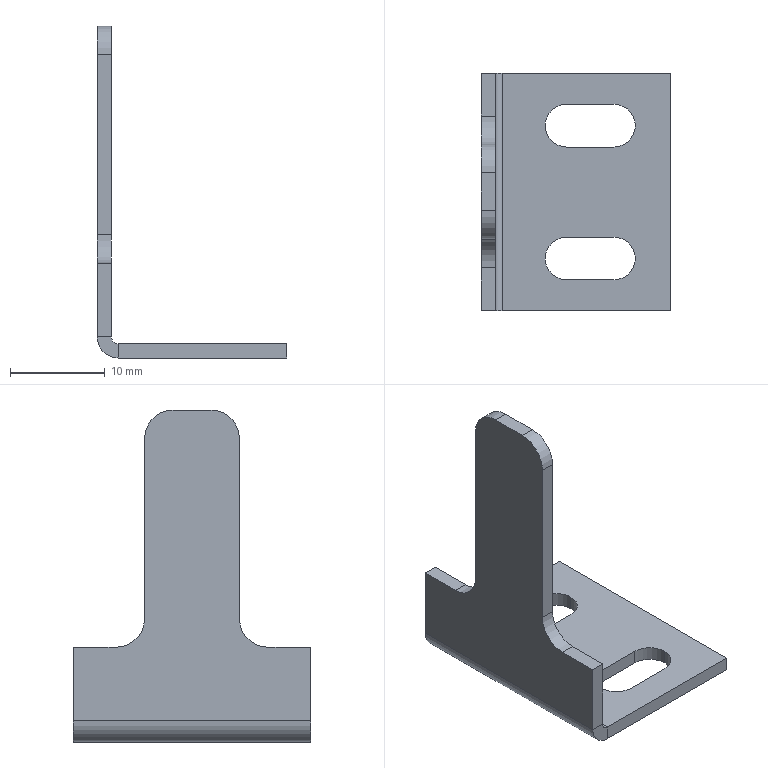Part | SolidWorks | features EdgeFlange 1, Fillet 1, FlatPattern 1, ICE 1, SMBaseFlange 1, SheetMetal 1 | 1 solid | 32 faces | box 20 x 25 x 35 mm | volume 1305 mm3 | plane 20 | cylinder 12 | commonest cylinder face diameters 4.5 x6 6 x4 1.473 x1 4.473 x1
STEP:
#1=CARTESIAN_POINT('',(6.25,-7.,-1.5));
#2=VERTEX_POINT('',#1);
#3=CARTESIAN_POINT('',(4.,-4.75,-1.5));
#4=VERTEX_POINT('',#3);
#5=CARTESIAN_POINT('',(4.,-7.,-1.5));
#6=DIRECTION('',(0.,0.,1.));
#7=DIRECTION('',(1.,0.,0.));
#8=AXIS2_PLACEMENT_3D('',#5,#6,#7);
#9=CIRCLE('',#8,2.25);
#10=EDGE_CURVE('',#2,#4,#9,.T.);
#11=ORIENTED_EDGE('',*,*,#10,.F.);
#12=CARTESIAN_POINT('',(6.25,-7.,0.));
#13=VERTEX_POINT('',#12);
#14=CARTESIAN_POINT('',(6.25,-7.,-1.5));
#15=DIRECTION('',(0.,0.,1.));
#16=VECTOR('',#15,1000.);
#17=LINE('',#14,#16);
#18=EDGE_CURVE('',#2,#13,#17,.T.);
#19=ORIENTED_EDGE('',*,*,#18,.T.);
#20=CARTESIAN_POINT('',(4.,-4.75,0.));
#21=VERTEX_POINT('',#20);
#22=CARTESIAN_POINT('',(4.,-7.,0.));
#23=DIRECTION('',(0.,0.,1.));
#24=DIRECTION('',(1.,0.,0.));
#25=AXIS2_PLACEMENT_3D('',#22,#23,#24);
#26=CIRCLE('',#25,2.25);
#27=EDGE_CURVE('',#13,#21,#26,.T.);
#28=ORIENTED_EDGE('',*,*,#27,.T.);
#29=CARTESIAN_POINT('',(4.,-4.75,-1.5));
#30=DIRECTION('',(0.,0.,1.));
#31=VECTOR('',#30,1000.);
#32=LINE('',#29,#31);
#33=EDGE_CURVE('',#4,#21,#32,.T.);
#34=ORIENTED_EDGE('',*,*,#33,.F.);
#35=EDGE_LOOP('',(#11,#19,#28,#34));
#36=FACE_OUTER_BOUND('',#35,.T.);
#37=CARTESIAN_POINT('',(4.,-7.,-1.5));
#38=DIRECTION('',(0.,0.,1.));
#39=DIRECTION('',(1.,0.,0.));
#40=AXIS2_PLACEMENT_3D('',#37,#38,#39);
#41=CYLINDRICAL_SURFACE('',#40,2.25);
#42=ADVANCED_FACE('',(#36),#41,.F.);
#43=CARTESIAN_POINT('',(6.25,7.,-1.5));
#44=VERTEX_POINT('',#43);
#45=CARTESIAN_POINT('',(4.,9.25,-1.5));
#46=VERTEX_POINT('',#45);
#47=CARTESIAN_POINT('',(4.,7.,-1.5));
#48=DIRECTION('',(0.,0.,1.));
#49=DIRECTION('',(1.,0.,0.));
#50=AXIS2_PLACEMENT_3D('',#47,#48,#49);
#51=CIRCLE('',#50,2.25);
#52=EDGE_CURVE('',#44,#46,#51,.T.);
#53=ORIENTED_EDGE('',*,*,#52,.F.);
#54=CARTESIAN_POINT('',(6.25,7.,0.));
#55=VERTEX_POINT('',#54);
#56=CARTESIAN_POINT('',(6.25,7.,-1.5));
#57=DIRECTION('',(0.,0.,1.));
#58=VECTOR('',#57,1000.);
#59=LINE('',#56,#58);
#60=EDGE_CURVE('',#44,#55,#59,.T.);
#61=ORIENTED_EDGE('',*,*,#60,.T.);
#62=CARTESIAN_POINT('',(4.,9.25,0.));
#63=VERTEX_POINT('',#62);
#64=CARTESIAN_POINT('',(4.,7.,0.));
#65=DIRECTION('',(0.,0.,1.));
#66=DIRECTION('',(1.,0.,0.));
#67=AXIS2_PLACEMENT_3D('',#64,#65,#66);
#68=CIRCLE('',#67,2.25);
#69=EDGE_CURVE('',#55,#63,#68,.T.);
#70=ORIENTED_EDGE('',*,*,#69,.T.);
#71=CARTESIAN_POINT('',(4.,9.25,-1.5));
#72=DIRECTION('',(0.,0.,1.));
#73=VECTOR('',#72,1000.);
#74=LINE('',#71,#73);
#75=EDGE_CURVE('',#46,#63,#74,.T.);
#76=ORIENTED_EDGE('',*,*,#75,.F.);
#77=EDGE_LOOP('',(#53,#61,#70,#76));
#78=FACE_OUTER_BOUND('',#77,.T.);
#79=CARTESIAN_POINT('',(4.,7.,-1.5));
#80=DIRECTION('',(0.,0.,1.));
#81=DIRECTION('',(1.,0.,0.));
#82=AXIS2_PLACEMENT_3D('',#79,#80,#81);
#83=CYLINDRICAL_SURFACE('',#82,2.25);
#84=ADVANCED_FACE('',(#78),#83,.F.);
#85=CARTESIAN_POINT('',(-7.763,-12.5,0.));
#86=VERTEX_POINT('',#85);
#87=CARTESIAN_POINT('',(10.,-12.5,0.));
#88=VERTEX_POINT('',#87);
#89=CARTESIAN_POINT('',(-10.,-12.5,0.));
#90=DIRECTION('',(1.,0.,0.));
#91=VECTOR('',#90,1000.);
#92=LINE('',#89,#91);
#93=EDGE_CURVE('',#86,#88,#92,.T.);
#94=ORIENTED_EDGE('',*,*,#93,.F.);
#95=CARTESIAN_POINT('',(-7.763,-12.5,-1.5));
#96=VERTEX_POINT('',#95);
#97=CARTESIAN_POINT('',(-7.763,-12.5,0.));
#98=DIRECTION('',(0.,0.,-1.));
#99=VECTOR('',#98,1000.);
#100=LINE('',#97,#99);
#101=EDGE_CURVE('',#86,#96,#100,.T.);
#102=ORIENTED_EDGE('',*,*,#101,.T.);
#103=CARTESIAN_POINT('',(10.,-12.5,-1.5));
#104=VERTEX_POINT('',#103);
#105=CARTESIAN_POINT('',(-10.,-12.5,-1.5));
#106=DIRECTION('',(1.,0.,0.));
#107=VECTOR('',#106,1000.);
#108=LINE('',#105,#107);
#109=EDGE_CURVE('',#96,#104,#108,.T.);
#110=ORIENTED_EDGE('',*,*,#109,.T.);
#111=CARTESIAN_POINT('',(10.,-12.5,-1.5));
#112=DIRECTION('',(0.,0.,1.));
#113=VECTOR('',#112,1000.);
#114=LINE('',#111,#113);
#115=EDGE_CURVE('',#104,#88,#114,.T.);
#116=ORIENTED_EDGE('',*,*,#115,.T.);
#117=EDGE_LOOP('',(#94,#102,#110,#116));
#118=FACE_OUTER_BOUND('',#117,.T.);
#119=CARTESIAN_POINT('',(-10.,-12.5,-1.5));
#120=DIRECTION('',(0.,-1.,0.));
#121=DIRECTION('',(0.,0.,-1.));
#122=AXIS2_PLACEMENT_3D('',#119,#120,#121);
#123=PLANE('',#122);
#124=ADVANCED_FACE('',(#118),#123,.T.);
#125=CARTESIAN_POINT('',(-1.,9.25,-1.5));
#126=VERTEX_POINT('',#125);
#127=CARTESIAN_POINT('',(-1.,9.25,-1.5));
#128=DIRECTION('',(-1.,0.,0.));
#129=VECTOR('',#128,1000.);
#130=LINE('',#127,#129);
#131=EDGE_CURVE('',#46,#126,#130,.T.);
#132=ORIENTED_EDGE('',*,*,#131,.T.);
#133=CARTESIAN_POINT('',(-1.,4.75,-1.5));
#134=VERTEX_POINT('',#133);
#135=CARTESIAN_POINT('',(-1.,7.,-1.5));
#136=DIRECTION('',(0.,0.,1.));
#137=DIRECTION('',(1.,0.,0.));
#138=AXIS2_PLACEMENT_3D('',#135,#136,#137);
#139=CIRCLE('',#138,2.25);
#140=EDGE_CURVE('',#126,#134,#139,.T.);
#141=ORIENTED_EDGE('',*,*,#140,.T.);
#142=CARTESIAN_POINT('',(4.,4.75,-1.5));
#143=VERTEX_POINT('',#142);
#144=CARTESIAN_POINT('',(-1.,4.75,-1.5));
#145=DIRECTION('',(1.,0.,0.));
#146=VECTOR('',#145,1000.);
#147=LINE('',#144,#146);
#148=EDGE_CURVE('',#134,#143,#147,.T.);
#149=ORIENTED_EDGE('',*,*,#148,.T.);
#150=CARTESIAN_POINT('',(4.,7.,-1.5));
#151=DIRECTION('',(0.,0.,1.));
#152=DIRECTION('',(1.,0.,0.));
#153=AXIS2_PLACEMENT_3D('',#150,#151,#152);
#154=CIRCLE('',#153,2.25);
#155=EDGE_CURVE('',#143,#44,#154,.T.);
#156=ORIENTED_EDGE('',*,*,#155,.T.);
#157=ORIENTED_EDGE('',*,*,#52,.T.);
#158=EDGE_LOOP('',(#132,#141,#149,#156,#157));
#159=FACE_BOUND('',#158,.T.);
#160=CARTESIAN_POINT('',(-1.,-4.75,-1.5));
#161=VERTEX_POINT('',#160);
#162=CARTESIAN_POINT('',(-1.,-4.75,-1.5));
#163=DIRECTION('',(-1.,0.,0.));
#164=VECTOR('',#163,1000.);
#165=LINE('',#162,#164);
#166=EDGE_CURVE('',#4,#161,#165,.T.);
#167=ORIENTED_EDGE('',*,*,#166,.T.);
#168=CARTESIAN_POINT('',(-1.,-9.25,-1.5));
#169=VERTEX_POINT('',#168);
#170=CARTESIAN_POINT('',(-1.,-7.,-1.5));
#171=DIRECTION('',(0.,0.,1.));
#172=DIRECTION('',(1.,0.,0.));
#173=AXIS2_PLACEMENT_3D('',#170,#171,#172);
#174=CIRCLE('',#173,2.25);
#175=EDGE_CURVE('',#161,#169,#174,.T.);
#176=ORIENTED_EDGE('',*,*,#175,.T.);
#177=CARTESIAN_POINT('',(4.,-9.25,-1.5));
#178=VERTEX_POINT('',#177);
#179=CARTESIAN_POINT('',(-1.,-9.25,-1.5));
#180=DIRECTION('',(1.,0.,0.));
#181=VECTOR('',#180,1000.);
#182=LINE('',#179,#181);
#183=EDGE_CURVE('',#169,#178,#182,.T.);
#184=ORIENTED_EDGE('',*,*,#183,.T.);
#185=CARTESIAN_POINT('',(4.,-7.,-1.5));
#186=DIRECTION('',(0.,0.,1.));
#187=DIRECTION('',(1.,0.,0.));
#188=AXIS2_PLACEMENT_3D('',#185,#186,#187);
#189=CIRCLE('',#188,2.25);
#190=EDGE_CURVE('',#178,#2,#189,.T.);
#191=ORIENTED_EDGE('',*,*,#190,.T.);
#192=ORIENTED_EDGE('',*,*,#10,.T.);
#193=EDGE_LOOP('',(#167,#176,#184,#191,#192));
#194=FACE_BOUND('',#193,.T.);
#195=CARTESIAN_POINT('',(-7.763,12.5,-1.5));
#196=VERTEX_POINT('',#195);
#197=CARTESIAN_POINT('',(-7.763,-12.5,-1.5));
#198=DIRECTION('',(0.,1.,0.));
#199=VECTOR('',#198,1000.);
#200=LINE('',#197,#199);
#201=EDGE_CURVE('',#96,#196,#200,.T.);
#202=ORIENTED_EDGE('',*,*,#201,.T.);
#203=CARTESIAN_POINT('',(10.,12.5,-1.5));
#204=VERTEX_POINT('',#203);
#205=CARTESIAN_POINT('',(-10.,12.5,-1.5));
#206=DIRECTION('',(-1.,0.,0.));
#207=VECTOR('',#206,1000.);
#208=LINE('',#205,#207);
#209=EDGE_CURVE('',#204,#196,#208,.T.);
#210=ORIENTED_EDGE('',*,*,#209,.F.);
#211=CARTESIAN_POINT('',(10.,12.5,-1.5));
#212=DIRECTION('',(0.,1.,0.));
#213=VECTOR('',#212,1000.);
#214=LINE('',#211,#213);
#215=EDGE_CURVE('',#104,#204,#214,.T.);
#216=ORIENTED_EDGE('',*,*,#215,.F.);
#217=ORIENTED_EDGE('',*,*,#109,.F.);
#218=EDGE_LOOP('',(#202,#210,#216,#217));
#219=FACE_OUTER_BOUND('',#218,.T.);
#220=CARTESIAN_POINT('',(0.,0.,-1.5));
#221=DIRECTION('',(0.,0.,1.));
#222=DIRECTION('',(1.,0.,0.));
#223=AXIS2_PLACEMENT_3D('',#220,#221,#222);
#224=PLANE('',#223);
#225=ADVANCED_FACE('',(#159,#194,#219),#224,.F.);
#226=CARTESIAN_POINT('',(-1.,9.25,0.));
#227=VERTEX_POINT('',#226);
#228=CARTESIAN_POINT('',(-1.,4.75,0.));
#229=VERTEX_POINT('',#228);
#230=CARTESIAN_POINT('',(-1.,7.,0.));
#231=DIRECTION('',(0.,0.,1.));
#232=DIRECTION('',(1.,0.,0.));
#233=AXIS2_PLACEMENT_3D('',#230,#231,#232);
#234=CIRCLE('',#233,2.25);
#235=EDGE_CURVE('',#227,#229,#234,.T.);
#236=ORIENTED_EDGE('',*,*,#235,.F.);
#237=CARTESIAN_POINT('',(-1.,9.25,0.));
#238=DIRECTION('',(-1.,0.,0.));
#239=VECTOR('',#238,1000.);
#240=LINE('',#237,#239);
#241=EDGE_CURVE('',#63,#227,#240,.T.);
#242=ORIENTED_EDGE('',*,*,#241,.F.);
#243=ORIENTED_EDGE('',*,*,#69,.F.);
#244=CARTESIAN_POINT('',(4.,4.75,0.));
#245=VERTEX_POINT('',#244);
#246=CARTESIAN_POINT('',(4.,7.,0.));
#247=DIRECTION('',(0.,0.,1.));
#248=DIRECTION('',(1.,0.,0.));
#249=AXIS2_PLACEMENT_3D('',#246,#247,#248);
#250=CIRCLE('',#249,2.25);
#251=EDGE_CURVE('',#245,#55,#250,.T.);
#252=ORIENTED_EDGE('',*,*,#251,.F.);
#253=CARTESIAN_POINT('',(-1.,4.75,0.));
#254=DIRECTION('',(1.,0.,0.));
#255=VECTOR('',#254,1000.);
#256=LINE('',#253,#255);
#257=EDGE_CURVE('',#229,#245,#256,.T.);
#258=ORIENTED_EDGE('',*,*,#257,.F.);
#259=EDGE_LOOP('',(#236,#242,#243,#252,#258));
#260=FACE_BOUND('',#259,.T.);
#261=CARTESIAN_POINT('',(-1.,-4.75,0.));
#262=VERTEX_POINT('',#261);
#263=CARTESIAN_POINT('',(-1.,-9.25,0.));
#264=VERTEX_POINT('',#263);
#265=CARTESIAN_POINT('',(-1.,-7.,0.));
#266=DIRECTION('',(0.,0.,1.));
#267=DIRECTION('',(1.,0.,0.));
#268=AXIS2_PLACEMENT_3D('',#265,#266,#267);
#269=CIRCLE('',#268,2.25);
#270=EDGE_CURVE('',#262,#264,#269,.T.);
#271=ORIENTED_EDGE('',*,*,#270,.F.);
#272=CARTESIAN_POINT('',(-1.,-4.75,0.));
#273=DIRECTION('',(-1.,0.,0.));
#274=VECTOR('',#273,1000.);
#275=LINE('',#272,#274);
#276=EDGE_CURVE('',#21,#262,#275,.T.);
#277=ORIENTED_EDGE('',*,*,#276,.F.);
#278=ORIENTED_EDGE('',*,*,#27,.F.);
#279=CARTESIAN_POINT('',(4.,-9.25,0.));
#280=VERTEX_POINT('',#279);
#281=CARTESIAN_POINT('',(4.,-7.,0.));
#282=DIRECTION('',(0.,0.,1.));
#283=DIRECTION('',(1.,0.,0.));
#284=AXIS2_PLACEMENT_3D('',#281,#282,#283);
#285=CIRCLE('',#284,2.25);
#286=EDGE_CURVE('',#280,#13,#285,.T.);
#287=ORIENTED_EDGE('',*,*,#286,.F.);
#288=CARTESIAN_POINT('',(-1.,-9.25,0.));
#289=DIRECTION('',(1.,0.,0.));
#290=VECTOR('',#289,1000.);
#291=LINE('',#288,#290);
#292=EDGE_CURVE('',#264,#280,#291,.T.);
#293=ORIENTED_EDGE('',*,*,#292,.F.);
#294=EDGE_LOOP('',(#271,#277,#278,#287,#293));
#295=FACE_BOUND('',#294,.T.);
#296=CARTESIAN_POINT('',(10.,12.5,0.));
#297=VERTEX_POINT('',#296);
#298=CARTESIAN_POINT('',(-7.763,12.5,0.));
#299=VERTEX_POINT('',#298);
#300=CARTESIAN_POINT('',(-10.,12.5,0.));
#301=DIRECTION('',(-1.,0.,0.));
#302=VECTOR('',#301,1000.);
#303=LINE('',#300,#302);
#304=EDGE_CURVE('',#297,#299,#303,.T.);
#305=ORIENTED_EDGE('',*,*,#304,.T.);
#306=CARTESIAN_POINT('',(-7.763,-12.5,0.));
#307=DIRECTION('',(0.,1.,0.));
#308=VECTOR('',#307,1000.);
#309=LINE('',#306,#308);
#310=EDGE_CURVE('',#86,#299,#309,.T.);
#311=ORIENTED_EDGE('',*,*,#310,.F.);
#312=ORIENTED_EDGE('',*,*,#93,.T.);
#313=CARTESIAN_POINT('',(10.,12.5,0.));
#314=DIRECTION('',(0.,1.,0.));
#315=VECTOR('',#314,1000.);
#316=LINE('',#313,#315);
#317=EDGE_CURVE('',#88,#297,#316,.T.);
#318=ORIENTED_EDGE('',*,*,#317,.T.);
#319=EDGE_LOOP('',(#305,#311,#312,#318));
#320=FACE_OUTER_BOUND('',#319,.T.);
#321=CARTESIAN_POINT('',(0.,0.,0.));
#322=DIRECTION('',(0.,0.,1.));
#323=DIRECTION('',(1.,0.,0.));
#324=AXIS2_PLACEMENT_3D('',#321,#322,#323);
#325=PLANE('',#324);
#326=ADVANCED_FACE('',(#260,#295,#320),#325,.T.);
#327=ORIENTED_EDGE('',*,*,#317,.F.);
#328=ORIENTED_EDGE('',*,*,#115,.F.);
#329=ORIENTED_EDGE('',*,*,#215,.T.);
#330=CARTESIAN_POINT('',(10.,12.5,-1.5));
#331=DIRECTION('',(0.,0.,1.));
#332=VECTOR('',#331,1000.);
#333=LINE('',#330,#332);
#334=EDGE_CURVE('',#204,#297,#333,.T.);
#335=ORIENTED_EDGE('',*,*,#334,.T.);
#336=EDGE_LOOP('',(#327,#328,#329,#335));
#337=FACE_OUTER_BOUND('',#336,.T.);
#338=CARTESIAN_POINT('',(10.,12.5,-1.5));
#339=DIRECTION('',(1.,0.,0.));
#340=DIRECTION('',(0.,1.,0.));
#341=AXIS2_PLACEMENT_3D('',#338,#339,#340);
#342=PLANE('',#341);
#343=ADVANCED_FACE('',(#337),#342,.T.);
#344=CARTESIAN_POINT('',(-7.763,12.5,0.));
#345=DIRECTION('',(0.,0.,-1.));
#346=VECTOR('',#345,1000.);
#347=LINE('',#344,#346);
#348=EDGE_CURVE('',#299,#196,#347,.T.);
#349=ORIENTED_EDGE('',*,*,#348,.F.);
#350=ORIENTED_EDGE('',*,*,#304,.F.);
#351=ORIENTED_EDGE('',*,*,#334,.F.);
#352=ORIENTED_EDGE('',*,*,#209,.T.);
#353=EDGE_LOOP('',(#349,#350,#351,#352));
#354=FACE_OUTER_BOUND('',#353,.T.);
#355=CARTESIAN_POINT('',(-10.,12.5,-1.5));
#356=DIRECTION('',(0.,1.,0.));
#357=DIRECTION('',(0.,0.,1.));
#358=AXIS2_PLACEMENT_3D('',#355,#356,#357);
#359=PLANE('',#358);
#360=ADVANCED_FACE('',(#354),#359,.T.);
#361=ORIENTED_EDGE('',*,*,#235,.T.);
#362=CARTESIAN_POINT('',(-1.,4.75,-1.5));
#363=DIRECTION('',(0.,0.,1.));
#364=VECTOR('',#363,1000.);
#365=LINE('',#362,#364);
#366=EDGE_CURVE('',#134,#229,#365,.T.);
#367=ORIENTED_EDGE('',*,*,#366,.F.);
#368=ORIENTED_EDGE('',*,*,#140,.F.);
#369=CARTESIAN_POINT('',(-1.,9.25,-1.5));
#370=DIRECTION('',(0.,0.,1.));
#371=VECTOR('',#370,1000.);
#372=LINE('',#369,#371);
#373=EDGE_CURVE('',#126,#227,#372,.T.);
#374=ORIENTED_EDGE('',*,*,#373,.T.);
#375=EDGE_LOOP('',(#361,#367,#368,#374));
#376=FACE_OUTER_BOUND('',#375,.T.);
#377=CARTESIAN_POINT('',(-1.,7.,-1.5));
#378=DIRECTION('',(0.,0.,1.));
#379=DIRECTION('',(1.,0.,0.));
#380=AXIS2_PLACEMENT_3D('',#377,#378,#379);
#381=CYLINDRICAL_SURFACE('',#380,2.25);
#382=ADVANCED_FACE('',(#376),#381,.F.);
#383=ORIENTED_EDGE('',*,*,#241,.T.);
#384=ORIENTED_EDGE('',*,*,#373,.F.);
#385=ORIENTED_EDGE('',*,*,#131,.F.);
#386=ORIENTED_EDGE('',*,*,#75,.T.);
#387=EDGE_LOOP('',(#383,#384,#385,#386));
#388=FACE_OUTER_BOUND('',#387,.T.);
#389=CARTESIAN_POINT('',(-1.,9.25,-1.5));
#390=DIRECTION('',(0.,1.,0.));
#391=DIRECTION('',(0.,0.,1.));
#392=AXIS2_PLACEMENT_3D('',#389,#390,#391);
#393=PLANE('',#392);
#394=ADVANCED_FACE('',(#388),#393,.F.);
#395=ORIENTED_EDGE('',*,*,#60,.F.);
#396=ORIENTED_EDGE('',*,*,#155,.F.);
#397=CARTESIAN_POINT('',(4.,4.75,-1.5));
#398=DIRECTION('',(0.,0.,1.));
#399=VECTOR('',#398,1000.);
#400=LINE('',#397,#399);
#401=EDGE_CURVE('',#143,#245,#400,.T.);
#402=ORIENTED_EDGE('',*,*,#401,.T.);
#403=ORIENTED_EDGE('',*,*,#251,.T.);
#404=EDGE_LOOP('',(#395,#396,#402,#403));
#405=FACE_OUTER_BOUND('',#404,.T.);
#406=CARTESIAN_POINT('',(4.,7.,-1.5));
#407=DIRECTION('',(0.,0.,1.));
#408=DIRECTION('',(1.,0.,0.));
#409=AXIS2_PLACEMENT_3D('',#406,#407,#408);
#410=CYLINDRICAL_SURFACE('',#409,2.25);
#411=ADVANCED_FACE('',(#405),#410,.F.);
#412=ORIENTED_EDGE('',*,*,#257,.T.);
#413=ORIENTED_EDGE('',*,*,#401,.F.);
#414=ORIENTED_EDGE('',*,*,#148,.F.);
#415=ORIENTED_EDGE('',*,*,#366,.T.);
#416=EDGE_LOOP('',(#412,#413,#414,#415));
#417=FACE_OUTER_BOUND('',#416,.T.);
#418=CARTESIAN_POINT('',(-1.,4.75,-1.5));
#419=DIRECTION('',(0.,-1.,0.));
#420=DIRECTION('',(0.,0.,-1.));
#421=AXIS2_PLACEMENT_3D('',#418,#419,#420);
#422=PLANE('',#421);
#423=ADVANCED_FACE('',(#417),#422,.F.);
#424=ORIENTED_EDGE('',*,*,#270,.T.);
#425=CARTESIAN_POINT('',(-1.,-9.25,-1.5));
#426=DIRECTION('',(0.,0.,1.));
#427=VECTOR('',#426,1000.);
#428=LINE('',#425,#427);
#429=EDGE_CURVE('',#169,#264,#428,.T.);
#430=ORIENTED_EDGE('',*,*,#429,.F.);
#431=ORIENTED_EDGE('',*,*,#175,.F.);
#432=CARTESIAN_POINT('',(-1.,-4.75,-1.5));
#433=DIRECTION('',(0.,0.,1.));
#434=VECTOR('',#433,1000.);
#435=LINE('',#432,#434);
#436=EDGE_CURVE('',#161,#262,#435,.T.);
#437=ORIENTED_EDGE('',*,*,#436,.T.);
#438=EDGE_LOOP('',(#424,#430,#431,#437));
#439=FACE_OUTER_BOUND('',#438,.T.);
#440=CARTESIAN_POINT('',(-1.,-7.,-1.5));
#441=DIRECTION('',(0.,0.,1.));
#442=DIRECTION('',(1.,0.,0.));
#443=AXIS2_PLACEMENT_3D('',#440,#441,#442);
#444=CYLINDRICAL_SURFACE('',#443,2.25);
#445=ADVANCED_FACE('',(#439),#444,.F.);
#446=ORIENTED_EDGE('',*,*,#276,.T.);
#447=ORIENTED_EDGE('',*,*,#436,.F.);
#448=ORIENTED_EDGE('',*,*,#166,.F.);
#449=ORIENTED_EDGE('',*,*,#33,.T.);
#450=EDGE_LOOP('',(#446,#447,#448,#449));
#451=FACE_OUTER_BOUND('',#450,.T.);
#452=CARTESIAN_POINT('',(-1.,-4.75,-1.5));
#453=DIRECTION('',(0.,1.,0.));
#454=DIRECTION('',(0.,0.,1.));
#455=AXIS2_PLACEMENT_3D('',#452,#453,#454);
#456=PLANE('',#455);
#457=ADVANCED_FACE('',(#451),#456,.F.);
#458=ORIENTED_EDGE('',*,*,#18,.F.);
#459=ORIENTED_EDGE('',*,*,#190,.F.);
#460=CARTESIAN_POINT('',(4.,-9.25,-1.5));
#461=DIRECTION('',(0.,0.,1.));
#462=VECTOR('',#461,1000.);
#463=LINE('',#460,#462);
#464=EDGE_CURVE('',#178,#280,#463,.T.);
#465=ORIENTED_EDGE('',*,*,#464,.T.);
#466=ORIENTED_EDGE('',*,*,#286,.T.);
#467=EDGE_LOOP('',(#458,#459,#465,#466));
#468=FACE_OUTER_BOUND('',#467,.T.);
#469=CARTESIAN_POINT('',(4.,-7.,-1.5));
#470=DIRECTION('',(0.,0.,1.));
#471=DIRECTION('',(1.,0.,0.));
#472=AXIS2_PLACEMENT_3D('',#469,#470,#471);
#473=CYLINDRICAL_SURFACE('',#472,2.25);
#474=ADVANCED_FACE('',(#468),#473,.F.);
#475=ORIENTED_EDGE('',*,*,#292,.T.);
#476=ORIENTED_EDGE('',*,*,#464,.F.);
#477=ORIENTED_EDGE('',*,*,#183,.F.);
#478=ORIENTED_EDGE('',*,*,#429,.T.);
#479=EDGE_LOOP('',(#475,#476,#477,#478));
#480=FACE_OUTER_BOUND('',#479,.T.);
#481=CARTESIAN_POINT('',(-1.,-9.25,-1.5));
#482=DIRECTION('',(0.,-1.,0.));
#483=DIRECTION('',(0.,0.,-1.));
#484=AXIS2_PLACEMENT_3D('',#481,#482,#483);
#485=PLANE('',#484);
#486=ADVANCED_FACE('',(#480),#485,.F.);
#487=CARTESIAN_POINT('',(-8.5,12.5,0.7366));
#488=VERTEX_POINT('',#487);
#489=CARTESIAN_POINT('',(-10.,12.5,0.7366));
#490=VERTEX_POINT('',#489);
#491=CARTESIAN_POINT('',(-10.,12.5,0.7366));
#492=DIRECTION('',(-1.,0.,0.));
#493=VECTOR('',#492,1000.);
#494=LINE('',#491,#493);
#495=EDGE_CURVE('',#488,#490,#494,.T.);
#496=ORIENTED_EDGE('',*,*,#495,.F.);
#497=CARTESIAN_POINT('',(-7.763,12.5,0.7366));
#498=DIRECTION('',(0.,1.,0.));
#499=DIRECTION('',(0.,0.,-1.));
#500=AXIS2_PLACEMENT_3D('',#497,#498,#499);
#501=CIRCLE('',#500,0.7366);
#502=EDGE_CURVE('',#299,#488,#501,.T.);
#503=ORIENTED_EDGE('',*,*,#502,.F.);
#504=ORIENTED_EDGE('',*,*,#348,.T.);
#505=CARTESIAN_POINT('',(-7.763,12.5,0.7366));
#506=DIRECTION('',(0.,1.,0.));
#507=DIRECTION('',(0.,0.,-1.));
#508=AXIS2_PLACEMENT_3D('',#505,#506,#507);
#509=CIRCLE('',#508,2.237);
#510=EDGE_CURVE('',#196,#490,#509,.T.);
#511=ORIENTED_EDGE('',*,*,#510,.T.);
#512=EDGE_LOOP('',(#496,#503,#504,#511));
#513=FACE_OUTER_BOUND('',#512,.T.);
#514=CARTESIAN_POINT('',(-7.763,12.5,0.7366));
#515=DIRECTION('',(0.,1.,0.));
#516=DIRECTION('',(0.,0.,1.));
#517=AXIS2_PLACEMENT_3D('',#514,#515,#516);
#518=PLANE('',#517);
#519=ADVANCED_FACE('',(#513),#518,.T.);
#520=CARTESIAN_POINT('',(-8.5,-12.5,0.7366));
#521=VERTEX_POINT('',#520);
#522=CARTESIAN_POINT('',(-7.763,-12.5,0.7366));
#523=DIRECTION('',(0.,-1.,0.));
#524=DIRECTION('',(0.,0.,-1.));
#525=AXIS2_PLACEMENT_3D('',#522,#523,#524);
#526=CIRCLE('',#525,0.7366);
#527=EDGE_CURVE('',#521,#86,#526,.T.);
#528=ORIENTED_EDGE('',*,*,#527,.F.);
#529=CARTESIAN_POINT('',(-10.,-12.5,0.7366));
#530=VERTEX_POINT('',#529);
#531=CARTESIAN_POINT('',(-8.5,-12.5,0.7366));
#532=DIRECTION('',(-1.,0.,0.));
#533=VECTOR('',#532,1000.);
#534=LINE('',#531,#533);
#535=EDGE_CURVE('',#521,#530,#534,.T.);
#536=ORIENTED_EDGE('',*,*,#535,.T.);
#537=CARTESIAN_POINT('',(-7.763,-12.5,0.7366));
#538=DIRECTION('',(0.,-1.,0.));
#539=DIRECTION('',(0.,0.,-1.));
#540=AXIS2_PLACEMENT_3D('',#537,#538,#539);
#541=CIRCLE('',#540,2.237);
#542=EDGE_CURVE('',#530,#96,#541,.T.);
#543=ORIENTED_EDGE('',*,*,#542,.T.);
#544=ORIENTED_EDGE('',*,*,#101,.F.);
#545=EDGE_LOOP('',(#528,#536,#543,#544));
#546=FACE_OUTER_BOUND('',#545,.T.);
#547=CARTESIAN_POINT('',(-7.763,-12.5,0.7366));
#548=DIRECTION('',(0.,1.,0.));
#549=DIRECTION('',(0.,0.,1.));
#550=AXIS2_PLACEMENT_3D('',#547,#548,#549);
#551=PLANE('',#550);
#552=ADVANCED_FACE('',(#546),#551,.F.);
#553=ORIENTED_EDGE('',*,*,#201,.F.);
#554=ORIENTED_EDGE('',*,*,#542,.F.);
#555=CARTESIAN_POINT('',(-10.,12.5,0.7366));
#556=DIRECTION('',(0.,1.,0.));
#557=VECTOR('',#556,1000.);
#558=LINE('',#555,#557);
#559=EDGE_CURVE('',#530,#490,#558,.T.);
#560=ORIENTED_EDGE('',*,*,#559,.T.);
#561=ORIENTED_EDGE('',*,*,#510,.F.);
#562=EDGE_LOOP('',(#553,#554,#560,#561));
#563=FACE_OUTER_BOUND('',#562,.T.);
#564=CARTESIAN_POINT('',(-7.763,-12.5,0.7366));
#565=DIRECTION('',(0.,-1.,0.));
#566=DIRECTION('',(-1.,0.,0.));
#567=AXIS2_PLACEMENT_3D('',#564,#565,#566);
#568=CYLINDRICAL_SURFACE('',#567,2.237);
#569=ADVANCED_FACE('',(#563),#568,.T.);
#570=ORIENTED_EDGE('',*,*,#310,.T.);
#571=ORIENTED_EDGE('',*,*,#502,.T.);
#572=CARTESIAN_POINT('',(-8.5,12.5,0.7366));
#573=DIRECTION('',(0.,-1.,0.));
#574=VECTOR('',#573,1000.);
#575=LINE('',#572,#574);
#576=EDGE_CURVE('',#488,#521,#575,.T.);
#577=ORIENTED_EDGE('',*,*,#576,.T.);
#578=ORIENTED_EDGE('',*,*,#527,.T.);
#579=EDGE_LOOP('',(#570,#571,#577,#578));
#580=FACE_OUTER_BOUND('',#579,.T.);
#581=CARTESIAN_POINT('',(-7.763,-12.5,0.7366));
#582=DIRECTION('',(0.,-1.,0.));
#583=DIRECTION('',(-1.,0.,0.));
#584=AXIS2_PLACEMENT_3D('',#581,#582,#583);
#585=CYLINDRICAL_SURFACE('',#584,0.7366);
#586=ADVANCED_FACE('',(#580),#585,.F.);
#587=CARTESIAN_POINT('',(-10.,12.5,8.5));
#588=VERTEX_POINT('',#587);
#589=CARTESIAN_POINT('',(-10.,12.5,0.));
#590=DIRECTION('',(0.,0.,-1.));
#591=VECTOR('',#590,1000.);
#592=LINE('',#589,#591);
#593=EDGE_CURVE('',#588,#490,#592,.T.);
#594=ORIENTED_EDGE('',*,*,#593,.F.);
#595=CARTESIAN_POINT('',(-8.5,12.5,8.5));
#596=VERTEX_POINT('',#595);
#597=CARTESIAN_POINT('',(0.,12.5,8.5));
#598=DIRECTION('',(-1.,0.,0.));
#599=VECTOR('',#598,1000.);
#600=LINE('',#597,#599);
#601=EDGE_CURVE('',#596,#588,#600,.T.);
#602=ORIENTED_EDGE('',*,*,#601,.F.);
#603=CARTESIAN_POINT('',(-8.5,12.5,0.));
#604=DIRECTION('',(0.,0.,-1.));
#605=VECTOR('',#604,1000.);
#606=LINE('',#603,#605);
#607=EDGE_CURVE('',#596,#488,#606,.T.);
#608=ORIENTED_EDGE('',*,*,#607,.T.);
#609=ORIENTED_EDGE('',*,*,#495,.T.);
#610=EDGE_LOOP('',(#594,#602,#608,#609));
#611=FACE_OUTER_BOUND('',#610,.T.);
#612=CARTESIAN_POINT('',(-10.,12.5,0.));
#613=DIRECTION('',(0.,-1.,0.));
#614=DIRECTION('',(1.,0.,0.));
#615=AXIS2_PLACEMENT_3D('',#612,#613,#614);
#616=PLANE('',#615);
#617=ADVANCED_FACE('',(#611),#616,.F.);
#618=CARTESIAN_POINT('',(-8.5,-12.5,8.5));
#619=VERTEX_POINT('',#618);
#620=CARTESIAN_POINT('',(-8.5,-12.5,33.5));
#621=DIRECTION('',(0.,0.,1.));
#622=VECTOR('',#621,1000.);
#623=LINE('',#620,#622);
#624=EDGE_CURVE('',#521,#619,#623,.T.);
#625=ORIENTED_EDGE('',*,*,#624,.T.);
#626=CARTESIAN_POINT('',(-10.,-12.5,8.5));
#627=VERTEX_POINT('',#626);
#628=CARTESIAN_POINT('',(0.,-12.5,8.5));
#629=DIRECTION('',(-1.,0.,0.));
#630=VECTOR('',#629,1000.);
#631=LINE('',#628,#630);
#632=EDGE_CURVE('',#619,#627,#631,.T.);
#633=ORIENTED_EDGE('',*,*,#632,.T.);
#634=CARTESIAN_POINT('',(-10.,-12.5,0.));
#635=DIRECTION('',(0.,0.,1.));
#636=VECTOR('',#635,1000.);
#637=LINE('',#634,#636);
#638=EDGE_CURVE('',#530,#627,#637,.T.);
#639=ORIENTED_EDGE('',*,*,#638,.F.);
#640=ORIENTED_EDGE('',*,*,#535,.F.);
#641=EDGE_LOOP('',(#625,#633,#639,#640));
#642=FACE_OUTER_BOUND('',#641,.T.);
#643=CARTESIAN_POINT('',(-10.,-12.5,33.5));
#644=DIRECTION('',(0.,1.,0.));
#645=DIRECTION('',(-1.,0.,0.));
#646=AXIS2_PLACEMENT_3D('',#643,#644,#645);
#647=PLANE('',#646);
#648=ADVANCED_FACE('',(#642),#647,.F.);
#649=CARTESIAN_POINT('',(-10.,-2.,33.5));
#650=VERTEX_POINT('',#649);
#651=CARTESIAN_POINT('',(-10.,2.,33.5));
#652=VERTEX_POINT('',#651);
#653=CARTESIAN_POINT('',(-10.,0.,33.5));
#654=DIRECTION('',(0.,1.,0.));
#655=VECTOR('',#654,1000.);
#656=LINE('',#653,#655);
#657=EDGE_CURVE('',#650,#652,#656,.T.);
#658=ORIENTED_EDGE('',*,*,#657,.T.);
#659=CARTESIAN_POINT('',(-10.,5.,30.5));
#660=VERTEX_POINT('',#659);
#661=CARTESIAN_POINT('',(-10.,2.,30.5));
#662=DIRECTION('',(-1.,0.,0.));
#663=DIRECTION('',(0.,0.,-1.));
#664=AXIS2_PLACEMENT_3D('',#661,#662,#663);
#665=CIRCLE('',#664,3.);
#666=EDGE_CURVE('',#652,#660,#665,.T.);
#667=ORIENTED_EDGE('',*,*,#666,.T.);
#668=CARTESIAN_POINT('',(-10.,5.,11.5));
#669=VERTEX_POINT('',#668);
#670=CARTESIAN_POINT('',(-10.,5.,33.5));
#671=DIRECTION('',(0.,0.,1.));
#672=VECTOR('',#671,1000.);
#673=LINE('',#670,#672);
#674=EDGE_CURVE('',#669,#660,#673,.T.);
#675=ORIENTED_EDGE('',*,*,#674,.F.);
#676=CARTESIAN_POINT('',(-10.,8.,8.5));
#677=VERTEX_POINT('',#676);
#678=CARTESIAN_POINT('',(-10.,8.,11.5));
#679=DIRECTION('',(1.,0.,0.));
#680=DIRECTION('',(0.,0.,-1.));
#681=AXIS2_PLACEMENT_3D('',#678,#679,#680);
#682=CIRCLE('',#681,3.);
#683=EDGE_CURVE('',#669,#677,#682,.T.);
#684=ORIENTED_EDGE('',*,*,#683,.T.);
#685=CARTESIAN_POINT('',(-10.,12.5,8.5));
#686=DIRECTION('',(0.,-1.,0.));
#687=VECTOR('',#686,1000.);
#688=LINE('',#685,#687);
#689=EDGE_CURVE('',#588,#677,#688,.T.);
#690=ORIENTED_EDGE('',*,*,#689,.F.);
#691=ORIENTED_EDGE('',*,*,#593,.T.);
#692=ORIENTED_EDGE('',*,*,#559,.F.);
#693=ORIENTED_EDGE('',*,*,#638,.T.);
#694=CARTESIAN_POINT('',(-10.,-8.,8.5));
#695=VERTEX_POINT('',#694);
#696=CARTESIAN_POINT('',(-10.,-12.5,8.5));
#697=DIRECTION('',(0.,-1.,0.));
#698=VECTOR('',#697,1000.);
#699=LINE('',#696,#698);
#700=EDGE_CURVE('',#695,#627,#699,.T.);
#701=ORIENTED_EDGE('',*,*,#700,.F.);
#702=CARTESIAN_POINT('',(-10.,-5.,11.5));
#703=VERTEX_POINT('',#702);
#704=CARTESIAN_POINT('',(-10.,-8.,11.5));
#705=DIRECTION('',(1.,0.,0.));
#706=DIRECTION('',(0.,0.,-1.));
#707=AXIS2_PLACEMENT_3D('',#704,#705,#706);
#708=CIRCLE('',#707,3.);
#709=EDGE_CURVE('',#695,#703,#708,.T.);
#710=ORIENTED_EDGE('',*,*,#709,.T.);
#711=CARTESIAN_POINT('',(-10.,-5.,30.5));
#712=VERTEX_POINT('',#711);
#713=CARTESIAN_POINT('',(-10.,-5.,33.5));
#714=DIRECTION('',(0.,0.,-1.));
#715=VECTOR('',#714,1000.);
#716=LINE('',#713,#715);
#717=EDGE_CURVE('',#712,#703,#716,.T.);
#718=ORIENTED_EDGE('',*,*,#717,.F.);
#719=CARTESIAN_POINT('',(-10.,-2.,30.5));
#720=DIRECTION('',(-1.,0.,0.));
#721=DIRECTION('',(0.,0.,-1.));
#722=AXIS2_PLACEMENT_3D('',#719,#720,#721);
#723=CIRCLE('',#722,3.);
#724=EDGE_CURVE('',#712,#650,#723,.T.);
#725=ORIENTED_EDGE('',*,*,#724,.T.);
#726=EDGE_LOOP('',(#658,#667,#675,#684,#690,#691,#692,#693,#701,#710,#718,#725));
#727=FACE_OUTER_BOUND('',#726,.T.);
#728=CARTESIAN_POINT('',(-10.,0.,0.));
#729=DIRECTION('',(1.,0.,0.));
#730=DIRECTION('',(0.,0.,-1.));
#731=AXIS2_PLACEMENT_3D('',#728,#729,#730);
#732=PLANE('',#731);
#733=ADVANCED_FACE('',(#727),#732,.F.);
#734=CARTESIAN_POINT('',(-8.5,5.,30.5));
#735=VERTEX_POINT('',#734);
#736=CARTESIAN_POINT('',(-8.5,5.,11.5));
#737=VERTEX_POINT('',#736);
#738=CARTESIAN_POINT('',(-8.5,5.,0.));
#739=DIRECTION('',(0.,0.,-1.));
#740=VECTOR('',#739,1000.);
#741=LINE('',#738,#740);
#742=EDGE_CURVE('',#735,#737,#741,.T.);
#743=ORIENTED_EDGE('',*,*,#742,.F.);
#744=CARTESIAN_POINT('',(-8.5,2.,33.5));
#745=VERTEX_POINT('',#744);
#746=CARTESIAN_POINT('',(-8.5,2.,30.5));
#747=DIRECTION('',(1.,0.,0.));
#748=DIRECTION('',(0.,0.,-1.));
#749=AXIS2_PLACEMENT_3D('',#746,#747,#748);
#750=CIRCLE('',#749,3.);
#751=EDGE_CURVE('',#735,#745,#750,.T.);
#752=ORIENTED_EDGE('',*,*,#751,.T.);
#753=CARTESIAN_POINT('',(-8.5,-2.,33.5));
#754=VERTEX_POINT('',#753);
#755=CARTESIAN_POINT('',(-8.5,12.5,33.5));
#756=DIRECTION('',(0.,1.,0.));
#757=VECTOR('',#756,1000.);
#758=LINE('',#755,#757);
#759=EDGE_CURVE('',#754,#745,#758,.T.);
#760=ORIENTED_EDGE('',*,*,#759,.F.);
#761=CARTESIAN_POINT('',(-8.5,-5.,30.5));
#762=VERTEX_POINT('',#761);
#763=CARTESIAN_POINT('',(-8.5,-2.,30.5));
#764=DIRECTION('',(1.,0.,0.));
#765=DIRECTION('',(0.,0.,-1.));
#766=AXIS2_PLACEMENT_3D('',#763,#764,#765);
#767=CIRCLE('',#766,3.);
#768=EDGE_CURVE('',#754,#762,#767,.T.);
#769=ORIENTED_EDGE('',*,*,#768,.T.);
#770=CARTESIAN_POINT('',(-8.5,-5.,11.5));
#771=VERTEX_POINT('',#770);
#772=CARTESIAN_POINT('',(-8.5,-5.,0.));
#773=DIRECTION('',(0.,0.,1.));
#774=VECTOR('',#773,1000.);
#775=LINE('',#772,#774);
#776=EDGE_CURVE('',#771,#762,#775,.T.);
#777=ORIENTED_EDGE('',*,*,#776,.F.);
#778=CARTESIAN_POINT('',(-8.5,-8.,8.5));
#779=VERTEX_POINT('',#778);
#780=CARTESIAN_POINT('',(-8.5,-8.,11.5));
#781=DIRECTION('',(-1.,0.,0.));
#782=DIRECTION('',(0.,0.,-1.));
#783=AXIS2_PLACEMENT_3D('',#780,#781,#782);
#784=CIRCLE('',#783,3.);
#785=EDGE_CURVE('',#771,#779,#784,.T.);
#786=ORIENTED_EDGE('',*,*,#785,.T.);
#787=CARTESIAN_POINT('',(-8.5,0.,8.5));
#788=DIRECTION('',(0.,1.,0.));
#789=VECTOR('',#788,1000.);
#790=LINE('',#787,#789);
#791=EDGE_CURVE('',#619,#779,#790,.T.);
#792=ORIENTED_EDGE('',*,*,#791,.F.);
#793=ORIENTED_EDGE('',*,*,#624,.F.);
#794=ORIENTED_EDGE('',*,*,#576,.F.);
#795=ORIENTED_EDGE('',*,*,#607,.F.);
#796=CARTESIAN_POINT('',(-8.5,8.,8.5));
#797=VERTEX_POINT('',#796);
#798=CARTESIAN_POINT('',(-8.5,0.,8.5));
#799=DIRECTION('',(0.,1.,0.));
#800=VECTOR('',#799,1000.);
#801=LINE('',#798,#800);
#802=EDGE_CURVE('',#797,#596,#801,.T.);
#803=ORIENTED_EDGE('',*,*,#802,.F.);
#804=CARTESIAN_POINT('',(-8.5,8.,11.5));
#805=DIRECTION('',(-1.,0.,0.));
#806=DIRECTION('',(0.,0.,-1.));
#807=AXIS2_PLACEMENT_3D('',#804,#805,#806);
#808=CIRCLE('',#807,3.);
#809=EDGE_CURVE('',#797,#737,#808,.T.);
#810=ORIENTED_EDGE('',*,*,#809,.T.);
#811=EDGE_LOOP('',(#743,#752,#760,#769,#777,#786,#792,#793,#794,#795,#803,#810));
#812=FACE_OUTER_BOUND('',#811,.T.);
#813=CARTESIAN_POINT('',(-8.5,0.,0.));
#814=DIRECTION('',(1.,0.,0.));
#815=DIRECTION('',(0.,0.,-1.));
#816=AXIS2_PLACEMENT_3D('',#813,#814,#815);
#817=PLANE('',#816);
#818=ADVANCED_FACE('',(#812),#817,.T.);
#819=ORIENTED_EDGE('',*,*,#759,.T.);
#820=CARTESIAN_POINT('',(-10.,2.,33.5));
#821=DIRECTION('',(-1.,0.,0.));
#822=VECTOR('',#821,1000.);
#823=LINE('',#820,#822);
#824=EDGE_CURVE('',#745,#652,#823,.T.);
#825=ORIENTED_EDGE('',*,*,#824,.T.);
#826=ORIENTED_EDGE('',*,*,#657,.F.);
#827=CARTESIAN_POINT('',(-10.,-2.,33.5));
#828=DIRECTION('',(1.,0.,0.));
#829=VECTOR('',#828,1000.);
#830=LINE('',#827,#829);
#831=EDGE_CURVE('',#650,#754,#830,.T.);
#832=ORIENTED_EDGE('',*,*,#831,.T.);
#833=EDGE_LOOP('',(#819,#825,#826,#832));
#834=FACE_OUTER_BOUND('',#833,.T.);
#835=CARTESIAN_POINT('',(-10.,12.5,33.5));
#836=DIRECTION('',(0.,0.,-1.));
#837=DIRECTION('',(-1.,0.,0.));
#838=AXIS2_PLACEMENT_3D('',#835,#836,#837);
#839=PLANE('',#838);
#840=ADVANCED_FACE('',(#834),#839,.F.);
#841=ORIENTED_EDGE('',*,*,#674,.T.);
#842=CARTESIAN_POINT('',(0.,5.,30.5));
#843=DIRECTION('',(1.,0.,0.));
#844=VECTOR('',#843,1000.);
#845=LINE('',#842,#844);
#846=EDGE_CURVE('',#660,#735,#845,.T.);
#847=ORIENTED_EDGE('',*,*,#846,.T.);
#848=ORIENTED_EDGE('',*,*,#742,.T.);
#849=CARTESIAN_POINT('',(-10.,5.,11.5));
#850=DIRECTION('',(-1.,0.,0.));
#851=VECTOR('',#850,1000.);
#852=LINE('',#849,#851);
#853=EDGE_CURVE('',#737,#669,#852,.T.);
#854=ORIENTED_EDGE('',*,*,#853,.T.);
#855=EDGE_LOOP('',(#841,#847,#848,#854));
#856=FACE_OUTER_BOUND('',#855,.T.);
#857=CARTESIAN_POINT('',(0.,5.,33.5));
#858=DIRECTION('',(0.,-1.,0.));
#859=DIRECTION('',(1.,0.,0.));
#860=AXIS2_PLACEMENT_3D('',#857,#858,#859);
#861=PLANE('',#860);
#862=ADVANCED_FACE('',(#856),#861,.F.);
#863=ORIENTED_EDGE('',*,*,#689,.T.);
#864=CARTESIAN_POINT('',(-8.5,8.,8.5));
#865=DIRECTION('',(1.,0.,0.));
#866=VECTOR('',#865,1000.);
#867=LINE('',#864,#866);
#868=EDGE_CURVE('',#677,#797,#867,.T.);
#869=ORIENTED_EDGE('',*,*,#868,.T.);
#870=ORIENTED_EDGE('',*,*,#802,.T.);
#871=ORIENTED_EDGE('',*,*,#601,.T.);
#872=EDGE_LOOP('',(#863,#869,#870,#871));
#873=FACE_OUTER_BOUND('',#872,.T.);
#874=CARTESIAN_POINT('',(0.,12.5,8.5));
#875=DIRECTION('',(0.,0.,-1.));
#876=DIRECTION('',(-1.,0.,0.));
#877=AXIS2_PLACEMENT_3D('',#874,#875,#876);
#878=PLANE('',#877);
#879=ADVANCED_FACE('',(#873),#878,.F.);
#880=ORIENTED_EDGE('',*,*,#791,.T.);
#881=CARTESIAN_POINT('',(-10.,-8.,8.5));
#882=DIRECTION('',(-1.,0.,0.));
#883=VECTOR('',#882,1000.);
#884=LINE('',#881,#883);
#885=EDGE_CURVE('',#779,#695,#884,.T.);
#886=ORIENTED_EDGE('',*,*,#885,.T.);
#887=ORIENTED_EDGE('',*,*,#700,.T.);
#888=ORIENTED_EDGE('',*,*,#632,.F.);
#889=EDGE_LOOP('',(#880,#886,#887,#888));
#890=FACE_OUTER_BOUND('',#889,.T.);
#891=CARTESIAN_POINT('',(0.,-12.5,8.5));
#892=DIRECTION('',(0.,0.,-1.));
#893=DIRECTION('',(-1.,0.,0.));
#894=AXIS2_PLACEMENT_3D('',#891,#892,#893);
#895=PLANE('',#894);
#896=ADVANCED_FACE('',(#890),#895,.F.);
#897=ORIENTED_EDGE('',*,*,#776,.T.);
#898=CARTESIAN_POINT('',(0.,-5.,30.5));
#899=DIRECTION('',(-1.,0.,0.));
#900=VECTOR('',#899,1000.);
#901=LINE('',#898,#900);
#902=EDGE_CURVE('',#762,#712,#901,.T.);
#903=ORIENTED_EDGE('',*,*,#902,.T.);
#904=ORIENTED_EDGE('',*,*,#717,.T.);
#905=CARTESIAN_POINT('',(-8.5,-5.,11.5));
#906=DIRECTION('',(1.,0.,0.));
#907=VECTOR('',#906,1000.);
#908=LINE('',#905,#907);
#909=EDGE_CURVE('',#703,#771,#908,.T.);
#910=ORIENTED_EDGE('',*,*,#909,.T.);
#911=EDGE_LOOP('',(#897,#903,#904,#910));
#912=FACE_OUTER_BOUND('',#911,.T.);
#913=CARTESIAN_POINT('',(0.,-5.,33.5));
#914=DIRECTION('',(0.,1.,0.));
#915=DIRECTION('',(-1.,0.,0.));
#916=AXIS2_PLACEMENT_3D('',#913,#914,#915);
#917=PLANE('',#916);
#918=ADVANCED_FACE('',(#912),#917,.F.);
#919=ORIENTED_EDGE('',*,*,#751,.F.);
#920=ORIENTED_EDGE('',*,*,#846,.F.);
#921=ORIENTED_EDGE('',*,*,#666,.F.);
#922=ORIENTED_EDGE('',*,*,#824,.F.);
#923=EDGE_LOOP('',(#919,#920,#921,#922));
#924=FACE_OUTER_BOUND('',#923,.T.);
#925=CARTESIAN_POINT('',(-10.,2.,30.5));
#926=DIRECTION('',(-1.,0.,0.));
#927=DIRECTION('',(0.,0.,1.));
#928=AXIS2_PLACEMENT_3D('',#925,#926,#927);
#929=CYLINDRICAL_SURFACE('',#928,3.);
#930=ADVANCED_FACE('',(#924),#929,.T.);
#931=ORIENTED_EDGE('',*,*,#724,.F.);
#932=ORIENTED_EDGE('',*,*,#902,.F.);
#933=ORIENTED_EDGE('',*,*,#768,.F.);
#934=ORIENTED_EDGE('',*,*,#831,.F.);
#935=EDGE_LOOP('',(#931,#932,#933,#934));
#936=FACE_OUTER_BOUND('',#935,.T.);
#937=CARTESIAN_POINT('',(-10.,-2.,30.5));
#938=DIRECTION('',(1.,0.,0.));
#939=DIRECTION('',(0.,0.,-1.));
#940=AXIS2_PLACEMENT_3D('',#937,#938,#939);
#941=CYLINDRICAL_SURFACE('',#940,3.);
#942=ADVANCED_FACE('',(#936),#941,.T.);
#943=ORIENTED_EDGE('',*,*,#785,.F.);
#944=ORIENTED_EDGE('',*,*,#909,.F.);
#945=ORIENTED_EDGE('',*,*,#709,.F.);
#946=ORIENTED_EDGE('',*,*,#885,.F.);
#947=EDGE_LOOP('',(#943,#944,#945,#946));
#948=FACE_OUTER_BOUND('',#947,.T.);
#949=CARTESIAN_POINT('',(0.,-8.,11.5));
#950=DIRECTION('',(1.,0.,0.));
#951=DIRECTION('',(0.,0.,-1.));
#952=AXIS2_PLACEMENT_3D('',#949,#950,#951);
#953=CYLINDRICAL_SURFACE('',#952,3.);
#954=ADVANCED_FACE('',(#948),#953,.F.);
#955=ORIENTED_EDGE('',*,*,#809,.F.);
#956=ORIENTED_EDGE('',*,*,#868,.F.);
#957=ORIENTED_EDGE('',*,*,#683,.F.);
#958=ORIENTED_EDGE('',*,*,#853,.F.);
#959=EDGE_LOOP('',(#955,#956,#957,#958));
#960=FACE_OUTER_BOUND('',#959,.T.);
#961=CARTESIAN_POINT('',(0.,8.,11.5));
#962=DIRECTION('',(1.,0.,0.));
#963=DIRECTION('',(0.,0.,-1.));
#964=AXIS2_PLACEMENT_3D('',#961,#962,#963);
#965=CYLINDRICAL_SURFACE('',#964,3.);
#966=ADVANCED_FACE('',(#960),#965,.F.);
#967=CLOSED_SHELL('',(#42,#84,#124,#225,#326,#343,#360,#382,#394,#411,#423,#445,#457,#474,#486,#519,#552,#569,#586,#617,#648,#733,#818,#840,#862,#879,#896,#918,#930,#942,#954,#966));
#968=MANIFOLD_SOLID_BREP('',#967);
#969=CARTESIAN_POINT('',(0.,0.,0.));
#970=DIRECTION('',(0.,0.,1.));
#971=DIRECTION('',(1.,0.,0.));
#972=AXIS2_PLACEMENT_3D('',#969,#970,#971);
#973=(LENGTH_UNIT()NAMED_UNIT(*)SI_UNIT(.MILLI.,.METRE.));
#974=UNCERTAINTY_MEASURE_WITH_UNIT(LENGTH_MEASURE(0.00001),#973,'','');
#975=(NAMED_UNIT(*)PLANE_ANGLE_UNIT()SI_UNIT($,.RADIAN.));
#976=(NAMED_UNIT(*)SI_UNIT($,.STERADIAN.)SOLID_ANGLE_UNIT());
#977=(GEOMETRIC_REPRESENTATION_CONTEXT(3)GLOBAL_UNCERTAINTY_ASSIGNED_CONTEXT((#974))GLOBAL_UNIT_ASSIGNED_CONTEXT((#973,#975,#976))REPRESENTATION_CONTEXT('',''));
#978=ADVANCED_BREP_SHAPE_REPRESENTATION('',(#968,#972),#977);